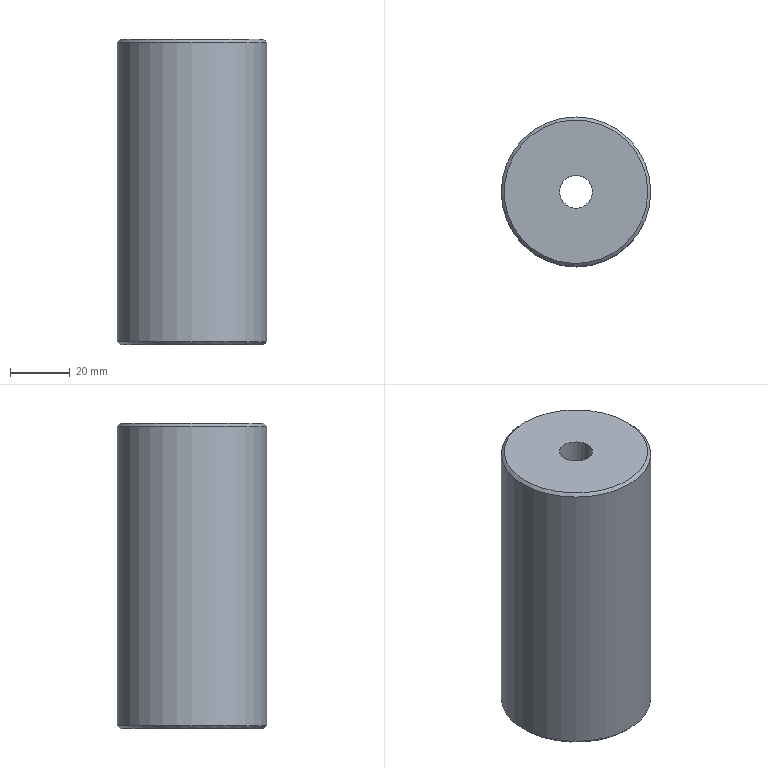Part | NX | features UB-1 2 | 1 solid | 8 faces | box 50 x 50 x 102 mm | volume 178228 mm3 | plane 3 | cylinder 3 | cone 2 | commonest cylinder face diameters 11.007 x1 18 x1 50 x1
STEP:
#1=CARTESIAN_POINT('',(2864.094,-666.122,960.716));
#2=VERTEX_POINT('',#1);
#3=CARTESIAN_POINT('',(2840.094,-666.122,960.716));
#4=DIRECTION('',(0.,0.,-1.));
#5=DIRECTION('',(1.,0.,0.));
#6=AXIS2_PLACEMENT_3D('',#3,#4,#5);
#7=CIRCLE('',#6,24.);
#8=EDGE_CURVE('',#2,#2,#7,.T.);
#9=ORIENTED_EDGE('',*,*,#8,.F.);
#10=EDGE_LOOP('',(#9));
#11=FACE_BOUND('',#10,.T.);
#12=CARTESIAN_POINT('',(2845.597,-666.122,960.716));
#13=VERTEX_POINT('',#12);
#14=CARTESIAN_POINT('',(2840.094,-666.122,960.716));
#15=DIRECTION('',(0.,0.,-1.));
#16=DIRECTION('',(1.,0.,0.));
#17=AXIS2_PLACEMENT_3D('',#14,#15,#16);
#18=CIRCLE('',#17,5.503);
#19=EDGE_CURVE('',#13,#13,#18,.F.);
#20=ORIENTED_EDGE('',*,*,#19,.F.);
#21=EDGE_LOOP('',(#20));
#22=FACE_BOUND('',#21,.T.);
#23=CARTESIAN_POINT('',(2840.094,-666.122,960.716));
#24=DIRECTION('',(0.,0.,1.));
#25=DIRECTION('',(-1.,0.,0.));
#26=AXIS2_PLACEMENT_3D('',#23,#24,#25);
#27=PLANE('',#26);
#28=ADVANCED_FACE('',(#11,#22),#27,.T.);
#29=CARTESIAN_POINT('',(2865.094,-666.122,959.716));
#30=VERTEX_POINT('',#29);
#31=CARTESIAN_POINT('',(2840.094,-666.122,959.716));
#32=DIRECTION('',(0.,0.,1.));
#33=DIRECTION('',(1.,0.,0.));
#34=AXIS2_PLACEMENT_3D('',#31,#32,#33);
#35=CIRCLE('',#34,25.);
#36=EDGE_CURVE('',#30,#30,#35,.T.);
#37=ORIENTED_EDGE('',*,*,#36,.F.);
#38=EDGE_LOOP('',(#37));
#39=FACE_BOUND('',#38,.T.);
#40=CARTESIAN_POINT('',(2865.094,-666.122,859.717));
#41=VERTEX_POINT('',#40);
#42=CARTESIAN_POINT('',(2840.094,-666.122,859.717));
#43=DIRECTION('',(0.,0.,-1.));
#44=DIRECTION('',(1.,0.,0.));
#45=AXIS2_PLACEMENT_3D('',#42,#43,#44);
#46=CIRCLE('',#45,25.);
#47=EDGE_CURVE('',#41,#41,#46,.T.);
#48=ORIENTED_EDGE('',*,*,#47,.F.);
#49=EDGE_LOOP('',(#48));
#50=FACE_BOUND('',#49,.T.);
#51=CARTESIAN_POINT('',(2840.094,-666.122,808.617));
#52=DIRECTION('',(0.,0.,1.));
#53=DIRECTION('',(-1.,0.,0.));
#54=AXIS2_PLACEMENT_3D('',#51,#52,#53);
#55=CYLINDRICAL_SURFACE('',#54,25.);
#56=ADVANCED_FACE('',(#39,#50),#55,.T.);
#57=CARTESIAN_POINT('',(2864.094,-666.122,858.717));
#58=VERTEX_POINT('',#57);
#59=CARTESIAN_POINT('',(2840.094,-666.122,858.717));
#60=DIRECTION('',(0.,0.,1.));
#61=DIRECTION('',(1.,0.,0.));
#62=AXIS2_PLACEMENT_3D('',#59,#60,#61);
#63=CIRCLE('',#62,24.);
#64=EDGE_CURVE('',#58,#58,#63,.T.);
#65=ORIENTED_EDGE('',*,*,#64,.F.);
#66=EDGE_LOOP('',(#65));
#67=FACE_BOUND('',#66,.T.);
#68=CARTESIAN_POINT('',(2831.094,-666.122,858.717));
#69=VERTEX_POINT('',#68);
#70=CARTESIAN_POINT('',(2840.094,-666.122,858.717));
#71=DIRECTION('',(0.,0.,-1.));
#72=DIRECTION('',(-1.,0.,0.));
#73=AXIS2_PLACEMENT_3D('',#70,#71,#72);
#74=CIRCLE('',#73,9.);
#75=EDGE_CURVE('',#69,#69,#74,.T.);
#76=ORIENTED_EDGE('',*,*,#75,.F.);
#77=EDGE_LOOP('',(#76));
#78=FACE_BOUND('',#77,.T.);
#79=CARTESIAN_POINT('',(2840.094,-666.122,858.717));
#80=DIRECTION('',(0.,0.,1.));
#81=DIRECTION('',(-1.,0.,0.));
#82=AXIS2_PLACEMENT_3D('',#79,#80,#81);
#83=PLANE('',#82);
#84=ADVANCED_FACE('',(#67,#78),#83,.F.);
#85=CARTESIAN_POINT('',(2845.597,-666.122,935.217));
#86=VERTEX_POINT('',#85);
#87=CARTESIAN_POINT('',(2840.094,-666.122,935.217));
#88=DIRECTION('',(0.,0.,-1.));
#89=DIRECTION('',(1.,0.,0.));
#90=AXIS2_PLACEMENT_3D('',#87,#88,#89);
#91=CIRCLE('',#90,5.503);
#92=EDGE_CURVE('',#86,#86,#91,.F.);
#93=ORIENTED_EDGE('',*,*,#92,.F.);
#94=EDGE_LOOP('',(#93));
#95=FACE_BOUND('',#94,.T.);
#96=ORIENTED_EDGE('',*,*,#19,.T.);
#97=EDGE_LOOP('',(#96));
#98=FACE_BOUND('',#97,.T.);
#99=CARTESIAN_POINT('',(2840.094,-666.122,965.217));
#100=DIRECTION('',(0.,0.,-1.));
#101=DIRECTION('',(1.,0.,0.));
#102=AXIS2_PLACEMENT_3D('',#99,#100,#101);
#103=CYLINDRICAL_SURFACE('',#102,5.503);
#104=ADVANCED_FACE('',(#95,#98),#103,.F.);
#105=CARTESIAN_POINT('',(2831.094,-666.122,935.217));
#106=VERTEX_POINT('',#105);
#107=CARTESIAN_POINT('',(2840.094,-666.122,935.217));
#108=DIRECTION('',(0.,0.,-1.));
#109=DIRECTION('',(-1.,0.,0.));
#110=AXIS2_PLACEMENT_3D('',#107,#108,#109);
#111=CIRCLE('',#110,9.);
#112=EDGE_CURVE('',#106,#106,#111,.T.);
#113=ORIENTED_EDGE('',*,*,#112,.T.);
#114=EDGE_LOOP('',(#113));
#115=FACE_BOUND('',#114,.T.);
#116=ORIENTED_EDGE('',*,*,#92,.T.);
#117=EDGE_LOOP('',(#116));
#118=FACE_BOUND('',#117,.T.);
#119=CARTESIAN_POINT('',(2840.094,-666.122,935.217));
#120=DIRECTION('',(0.,0.,1.));
#121=DIRECTION('',(-1.,0.,0.));
#122=AXIS2_PLACEMENT_3D('',#119,#120,#121);
#123=PLANE('',#122);
#124=ADVANCED_FACE('',(#115,#118),#123,.F.);
#125=ORIENTED_EDGE('',*,*,#75,.T.);
#126=EDGE_LOOP('',(#125));
#127=FACE_BOUND('',#126,.T.);
#128=ORIENTED_EDGE('',*,*,#112,.F.);
#129=EDGE_LOOP('',(#128));
#130=FACE_BOUND('',#129,.T.);
#131=CARTESIAN_POINT('',(2840.094,-666.122,935.217));
#132=DIRECTION('',(0.,0.,-1.));
#133=DIRECTION('',(1.,0.,0.));
#134=AXIS2_PLACEMENT_3D('',#131,#132,#133);
#135=CYLINDRICAL_SURFACE('',#134,9.);
#136=ADVANCED_FACE('',(#127,#130),#135,.F.);
#137=ORIENTED_EDGE('',*,*,#8,.T.);
#138=EDGE_LOOP('',(#137));
#139=FACE_BOUND('',#138,.T.);
#140=ORIENTED_EDGE('',*,*,#36,.T.);
#141=EDGE_LOOP('',(#140));
#142=FACE_BOUND('',#141,.T.);
#143=CARTESIAN_POINT('',(2840.094,-666.122,959.716));
#144=DIRECTION('',(0.,0.,-1.));
#145=DIRECTION('',(1.,0.,0.));
#146=AXIS2_PLACEMENT_3D('',#143,#144,#145);
#147=CONICAL_SURFACE('',#146,25.,0.7854);
#148=ADVANCED_FACE('',(#139,#142),#147,.T.);
#149=ORIENTED_EDGE('',*,*,#47,.T.);
#150=EDGE_LOOP('',(#149));
#151=FACE_BOUND('',#150,.T.);
#152=ORIENTED_EDGE('',*,*,#64,.T.);
#153=EDGE_LOOP('',(#152));
#154=FACE_BOUND('',#153,.T.);
#155=CARTESIAN_POINT('',(2840.094,-666.122,858.717));
#156=DIRECTION('',(0.,0.,1.));
#157=DIRECTION('',(-1.,0.,0.));
#158=AXIS2_PLACEMENT_3D('',#155,#156,#157);
#159=CONICAL_SURFACE('',#158,24.,0.7854);
#160=ADVANCED_FACE('',(#151,#154),#159,.T.);
#161=CLOSED_SHELL('',(#28,#56,#84,#104,#124,#136,#148,#160));
#162=MANIFOLD_SOLID_BREP('',#161);
#163=(LENGTH_UNIT()NAMED_UNIT(*)SI_UNIT(.MILLI.,.METRE.));
#164=UNCERTAINTY_MEASURE_WITH_UNIT(LENGTH_MEASURE(0.00001),#163,'','');
#165=(NAMED_UNIT(*)PLANE_ANGLE_UNIT()SI_UNIT($,.RADIAN.));
#166=(NAMED_UNIT(*)SI_UNIT($,.STERADIAN.)SOLID_ANGLE_UNIT());
#167=(GEOMETRIC_REPRESENTATION_CONTEXT(3)GLOBAL_UNCERTAINTY_ASSIGNED_CONTEXT((#164))GLOBAL_UNIT_ASSIGNED_CONTEXT((#163,#165,#166))REPRESENTATION_CONTEXT('',''));
#168=ADVANCED_BREP_SHAPE_REPRESENTATION('',(#162),#167);